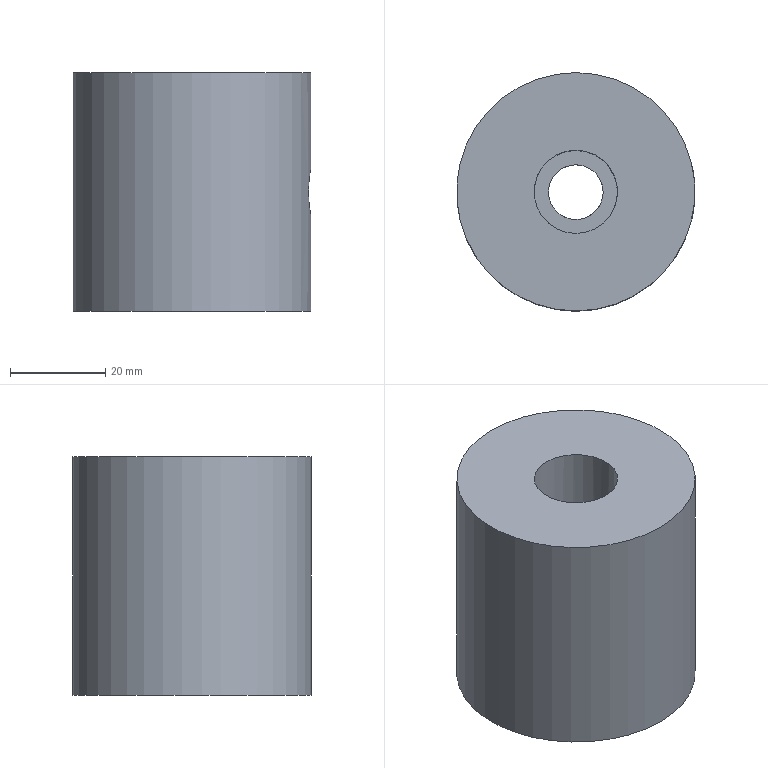Part | NX | features solid 2 | 1 solid | 9 faces | box 50 x 50 x 50 mm | volume 86329 mm3 | cylinder 5 | plane 4 | commonest cylinder face diameters 6 x1 10 x1 11.5 x1 17.5 x1 50 x1
STEP:
#1=CARTESIAN_POINT('',(1060.,273.75,70.));
#2=VERTEX_POINT('',#1);
#3=CARTESIAN_POINT('',(1060.,265.,70.));
#4=DIRECTION('',(0.,0.,-1.));
#5=DIRECTION('',(0.,1.,0.));
#6=AXIS2_PLACEMENT_3D('',#3,#4,#5);
#7=CIRCLE('',#6,8.75);
#8=EDGE_CURVE('',#2,#2,#7,.T.);
#9=ORIENTED_EDGE('',*,*,#8,.T.);
#10=EDGE_LOOP('',(#9));
#11=FACE_BOUND('',#10,.T.);
#12=CARTESIAN_POINT('',(1060.,290.,70.));
#13=VERTEX_POINT('',#12);
#14=CARTESIAN_POINT('',(1060.,265.,70.));
#15=DIRECTION('',(0.,0.,-1.));
#16=DIRECTION('',(0.,1.,0.));
#17=AXIS2_PLACEMENT_3D('',#14,#15,#16);
#18=CIRCLE('',#17,25.);
#19=EDGE_CURVE('',#13,#13,#18,.F.);
#20=ORIENTED_EDGE('',*,*,#19,.T.);
#21=EDGE_LOOP('',(#20));
#22=FACE_BOUND('',#21,.T.);
#23=CARTESIAN_POINT('',(1060.,265.,70.));
#24=DIRECTION('',(0.,0.,1.));
#25=DIRECTION('',(1.,0.,0.));
#26=AXIS2_PLACEMENT_3D('',#23,#24,#25);
#27=PLANE('',#26);
#28=ADVANCED_FACE('',(#11,#22),#27,.T.);
#29=CARTESIAN_POINT('',(1060.,290.,20.));
#30=VERTEX_POINT('',#29);
#31=CARTESIAN_POINT('',(1060.,265.,20.));
#32=DIRECTION('',(0.,0.,-1.));
#33=DIRECTION('',(0.,1.,0.));
#34=AXIS2_PLACEMENT_3D('',#31,#32,#33);
#35=CIRCLE('',#34,25.);
#36=EDGE_CURVE('',#30,#30,#35,.T.);
#37=ORIENTED_EDGE('',*,*,#36,.T.);
#38=EDGE_LOOP('',(#37));
#39=FACE_BOUND('',#38,.T.);
#40=CARTESIAN_POINT('',(1060.,270.75,20.));
#41=VERTEX_POINT('',#40);
#42=CARTESIAN_POINT('',(1060.,265.,20.));
#43=DIRECTION('',(0.,0.,-1.));
#44=DIRECTION('',(0.,1.,0.));
#45=AXIS2_PLACEMENT_3D('',#42,#43,#44);
#46=CIRCLE('',#45,5.75);
#47=EDGE_CURVE('',#41,#41,#46,.T.);
#48=ORIENTED_EDGE('',*,*,#47,.F.);
#49=EDGE_LOOP('',(#48));
#50=FACE_BOUND('',#49,.T.);
#51=CARTESIAN_POINT('',(1060.,265.,20.));
#52=DIRECTION('',(0.,0.,1.));
#53=DIRECTION('',(1.,0.,0.));
#54=AXIS2_PLACEMENT_3D('',#51,#52,#53);
#55=PLANE('',#54);
#56=ADVANCED_FACE('',(#39,#50),#55,.F.);
#57=CARTESIAN_POINT('',(1068.75,265.,25.));
#58=VERTEX_POINT('',#57);
#59=CARTESIAN_POINT('',(1060.,265.,25.));
#60=DIRECTION('',(0.,0.,-1.));
#61=DIRECTION('',(1.,0.,0.));
#62=AXIS2_PLACEMENT_3D('',#59,#60,#61);
#63=CIRCLE('',#62,8.75);
#64=EDGE_CURVE('',#58,#58,#63,.T.);
#65=ORIENTED_EDGE('',*,*,#64,.F.);
#66=EDGE_LOOP('',(#65));
#67=FACE_BOUND('',#66,.T.);
#68=CARTESIAN_POINT('',(1065.75,265.,25.));
#69=VERTEX_POINT('',#68);
#70=CARTESIAN_POINT('',(1060.,265.,25.));
#71=DIRECTION('',(0.,0.,-1.));
#72=DIRECTION('',(1.,0.,0.));
#73=AXIS2_PLACEMENT_3D('',#70,#71,#72);
#74=CIRCLE('',#73,5.75);
#75=EDGE_CURVE('',#69,#69,#74,.T.);
#76=ORIENTED_EDGE('',*,*,#75,.T.);
#77=EDGE_LOOP('',(#76));
#78=FACE_BOUND('',#77,.T.);
#79=CARTESIAN_POINT('',(1060.,265.,25.));
#80=DIRECTION('',(0.,0.,1.));
#81=DIRECTION('',(1.,0.,0.));
#82=AXIS2_PLACEMENT_3D('',#79,#80,#81);
#83=PLANE('',#82);
#84=ADVANCED_FACE('',(#67,#78),#83,.T.);
#85=ORIENTED_EDGE('',*,*,#19,.F.);
#86=EDGE_LOOP('',(#85));
#87=FACE_BOUND('',#86,.T.);
#88=CARTESIAN_POINT('',(1084.978,263.945,40.113));
#89=VERTEX_POINT('',#88);
#90=CARTESIAN_POINT('',(1084.593,260.344,41.995));
#91=CARTESIAN_POINT('',(1085.092,263.829,39.583));
#92=CARTESIAN_POINT('',(1084.905,268.011,40.35));
#93=CARTESIAN_POINT('',(1084.402,270.414,43.824));
#94=CARTESIAN_POINT('',(1084.594,269.653,48.01));
#95=CARTESIAN_POINT('',(1085.092,266.173,50.414));
#96=CARTESIAN_POINT('',(1084.906,261.995,49.656));
#97=CARTESIAN_POINT('',(1084.402,259.585,46.174));
#98=CARTESIAN_POINT('',(1084.593,260.344,41.995));
#99=CARTESIAN_POINT('',(1085.092,263.829,39.583));
#100=CARTESIAN_POINT('',(1084.905,268.011,40.35));
#101=B_SPLINE_CURVE_WITH_KNOTS('',3,(#90,#91,#92,#93,#94,#95,#96,#97,#98,#99,#100),.UNSPECIFIED.,.T.,.F.,(1,1,1,1,1,1,1,1,1,1,1,1,1,1,1),(-0.01175,-0.007836,-0.003918,0.,0.003918,0.007836,0.01175,0.01567,0.01959,0.02351,0.02743,0.03134,0.03526,0.03918,0.0431),.UNSPECIFIED.);
#102=EDGE_CURVE('',#89,#89,#101,.T.);
#103=ORIENTED_EDGE('',*,*,#102,.F.);
#104=EDGE_LOOP('',(#103));
#105=FACE_BOUND('',#104,.T.);
#106=ORIENTED_EDGE('',*,*,#36,.F.);
#107=EDGE_LOOP('',(#106));
#108=FACE_BOUND('',#107,.T.);
#109=CARTESIAN_POINT('',(1060.,265.,85.));
#110=DIRECTION('',(0.,0.,-1.));
#111=DIRECTION('',(-1.,0.,0.));
#112=AXIS2_PLACEMENT_3D('',#109,#110,#111);
#113=CYLINDRICAL_SURFACE('',#112,25.);
#114=ADVANCED_FACE('',(#87,#105,#108),#113,.T.);
#115=CARTESIAN_POINT('',(1068.75,265.,48.));
#116=VERTEX_POINT('',#115);
#117=CARTESIAN_POINT('',(1068.493,267.351,47.35));
#118=CARTESIAN_POINT('',(1068.879,265.,48.325));
#119=CARTESIAN_POINT('',(1068.493,262.648,47.348));
#120=CARTESIAN_POINT('',(1068.083,261.676,45.004));
#121=CARTESIAN_POINT('',(1068.493,262.65,42.648));
#122=CARTESIAN_POINT('',(1068.878,264.998,41.676));
#123=CARTESIAN_POINT('',(1068.493,267.351,42.649));
#124=CARTESIAN_POINT('',(1068.083,268.324,45.));
#125=CARTESIAN_POINT('',(1068.493,267.351,47.35));
#126=CARTESIAN_POINT('',(1068.879,265.,48.325));
#127=CARTESIAN_POINT('',(1068.493,262.648,47.348));
#128=B_SPLINE_CURVE_WITH_KNOTS('',3,(#117,#118,#119,#120,#121,#122,#123,#124,#125,#126,#127),.UNSPECIFIED.,.T.,.F.,(1,1,1,1,1,1,1,1,1,1,1,1,1,1,1),(-0.007088,-0.004725,-0.002363,0.,0.002363,0.004725,0.007088,0.00945,0.01181,0.01418,0.01654,0.0189,0.02126,0.02363,0.02599),.UNSPECIFIED.);
#129=EDGE_CURVE('',#116,#116,#128,.T.);
#130=ORIENTED_EDGE('',*,*,#129,.T.);
#131=EDGE_LOOP('',(#130));
#132=FACE_BOUND('',#131,.T.);
#133=ORIENTED_EDGE('',*,*,#8,.F.);
#134=EDGE_LOOP('',(#133));
#135=FACE_BOUND('',#134,.T.);
#136=ORIENTED_EDGE('',*,*,#64,.T.);
#137=EDGE_LOOP('',(#136));
#138=FACE_BOUND('',#137,.T.);
#139=CARTESIAN_POINT('',(1060.,265.,85.));
#140=DIRECTION('',(0.,0.,-1.));
#141=DIRECTION('',(-1.,0.,0.));
#142=AXIS2_PLACEMENT_3D('',#139,#140,#141);
#143=CYLINDRICAL_SURFACE('',#142,8.75);
#144=ADVANCED_FACE('',(#132,#135,#138),#143,.F.);
#145=ORIENTED_EDGE('',*,*,#75,.F.);
#146=EDGE_LOOP('',(#145));
#147=FACE_BOUND('',#146,.T.);
#148=ORIENTED_EDGE('',*,*,#47,.T.);
#149=EDGE_LOOP('',(#148));
#150=FACE_BOUND('',#149,.T.);
#151=CARTESIAN_POINT('',(1060.,265.,25.));
#152=DIRECTION('',(0.,0.,-1.));
#153=DIRECTION('',(-1.,0.,0.));
#154=AXIS2_PLACEMENT_3D('',#151,#152,#153);
#155=CYLINDRICAL_SURFACE('',#154,5.75);
#156=ADVANCED_FACE('',(#147,#150),#155,.F.);
#157=CARTESIAN_POINT('',(1084.,265.,50.));
#158=VERTEX_POINT('',#157);
#159=CARTESIAN_POINT('',(1084.,265.,45.));
#160=DIRECTION('',(-1.,0.,0.));
#161=DIRECTION('',(0.,0.,1.));
#162=AXIS2_PLACEMENT_3D('',#159,#160,#161);
#163=CIRCLE('',#162,5.);
#164=EDGE_CURVE('',#158,#158,#163,.T.);
#165=ORIENTED_EDGE('',*,*,#164,.T.);
#166=EDGE_LOOP('',(#165));
#167=FACE_BOUND('',#166,.T.);
#168=ORIENTED_EDGE('',*,*,#102,.T.);
#169=EDGE_LOOP('',(#168));
#170=FACE_BOUND('',#169,.T.);
#171=CARTESIAN_POINT('',(1090.5,265.,45.));
#172=DIRECTION('',(1.,0.,0.));
#173=DIRECTION('',(0.,0.,-1.));
#174=AXIS2_PLACEMENT_3D('',#171,#172,#173);
#175=CYLINDRICAL_SURFACE('',#174,5.);
#176=ADVANCED_FACE('',(#167,#170),#175,.F.);
#177=CARTESIAN_POINT('',(1084.,265.,48.));
#178=VERTEX_POINT('',#177);
#179=CARTESIAN_POINT('',(1084.,265.,45.));
#180=DIRECTION('',(-1.,0.,0.));
#181=DIRECTION('',(0.,0.,1.));
#182=AXIS2_PLACEMENT_3D('',#179,#180,#181);
#183=CIRCLE('',#182,3.);
#184=EDGE_CURVE('',#178,#178,#183,.F.);
#185=ORIENTED_EDGE('',*,*,#184,.F.);
#186=EDGE_LOOP('',(#185));
#187=FACE_BOUND('',#186,.T.);
#188=ORIENTED_EDGE('',*,*,#164,.F.);
#189=EDGE_LOOP('',(#188));
#190=FACE_BOUND('',#189,.T.);
#191=CARTESIAN_POINT('',(1084.,265.,45.));
#192=DIRECTION('',(1.,0.,0.));
#193=DIRECTION('',(0.,0.,-1.));
#194=AXIS2_PLACEMENT_3D('',#191,#192,#193);
#195=PLANE('',#194);
#196=ADVANCED_FACE('',(#187,#190),#195,.T.);
#197=ORIENTED_EDGE('',*,*,#129,.F.);
#198=EDGE_LOOP('',(#197));
#199=FACE_BOUND('',#198,.T.);
#200=ORIENTED_EDGE('',*,*,#184,.T.);
#201=EDGE_LOOP('',(#200));
#202=FACE_BOUND('',#201,.T.);
#203=CARTESIAN_POINT('',(1090.5,265.,45.));
#204=DIRECTION('',(-1.,0.,0.));
#205=DIRECTION('',(0.,0.,1.));
#206=AXIS2_PLACEMENT_3D('',#203,#204,#205);
#207=CYLINDRICAL_SURFACE('',#206,3.);
#208=ADVANCED_FACE('',(#199,#202),#207,.F.);
#209=CLOSED_SHELL('',(#28,#56,#84,#114,#144,#156,#176,#196,#208));
#210=MANIFOLD_SOLID_BREP('',#209);
#211=(LENGTH_UNIT()NAMED_UNIT(*)SI_UNIT(.MILLI.,.METRE.));
#212=UNCERTAINTY_MEASURE_WITH_UNIT(LENGTH_MEASURE(0.0508),#211,'','');
#213=(NAMED_UNIT(*)PLANE_ANGLE_UNIT()SI_UNIT($,.RADIAN.));
#214=(NAMED_UNIT(*)SI_UNIT($,.STERADIAN.)SOLID_ANGLE_UNIT());
#215=(GEOMETRIC_REPRESENTATION_CONTEXT(3)GLOBAL_UNCERTAINTY_ASSIGNED_CONTEXT((#212))GLOBAL_UNIT_ASSIGNED_CONTEXT((#211,#213,#214))REPRESENTATION_CONTEXT('',''));
#216=ADVANCED_BREP_SHAPE_REPRESENTATION('',(#210),#215);